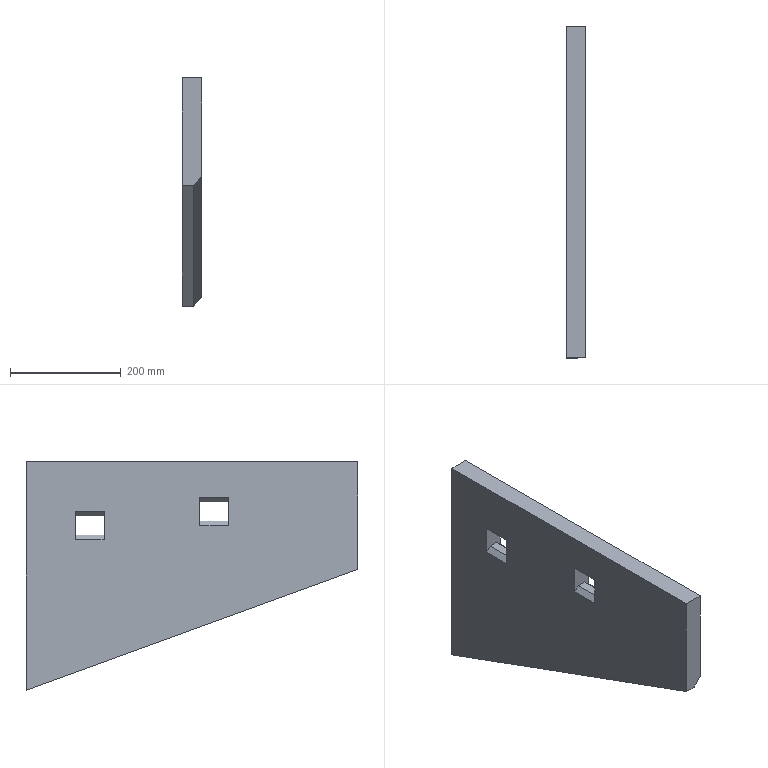Part | SolidWorks | features ICE 2, Chamfer 1, Extrusion 1 | 1 solid | 23 faces | box 35 x 600 x 413 mm | volume 6164844 mm3 | plane 23
STEP:
#1=CARTESIAN_POINT('',(2.5,-300.,-194.618));
#2=VERTEX_POINT('',#1);
#3=CARTESIAN_POINT('',(-17.5,-300.,-194.618));
#4=VERTEX_POINT('',#3);
#5=CARTESIAN_POINT('',(17.5,-300.,-194.618));
#6=DIRECTION('',(-1.,0.,0.));
#7=VECTOR('',#6,1000.);
#8=LINE('',#5,#7);
#9=EDGE_CURVE('',#2,#4,#8,.T.);
#10=ORIENTED_EDGE('',*,*,#9,.F.);
#11=CARTESIAN_POINT('',(17.5,-300.,-178.655));
#12=VERTEX_POINT('',#11);
#13=CARTESIAN_POINT('',(-20.187,-300.,-218.761));
#14=DIRECTION('',(0.6848,0.,0.7287));
#15=VECTOR('',#14,1000.);
#16=LINE('',#13,#15);
#17=EDGE_CURVE('',#2,#12,#16,.T.);
#18=ORIENTED_EDGE('',*,*,#17,.T.);
#19=CARTESIAN_POINT('',(17.5,-300.,0.));
#20=VERTEX_POINT('',#19);
#21=CARTESIAN_POINT('',(17.5,-300.,-194.618));
#22=DIRECTION('',(0.,0.,-1.));
#23=VECTOR('',#22,1000.);
#24=LINE('',#21,#23);
#25=EDGE_CURVE('',#20,#12,#24,.T.);
#26=ORIENTED_EDGE('',*,*,#25,.F.);
#27=CARTESIAN_POINT('',(-17.5,-300.,0.));
#28=VERTEX_POINT('',#27);
#29=CARTESIAN_POINT('',(17.5,-300.,0.));
#30=DIRECTION('',(-1.,0.,0.));
#31=VECTOR('',#30,1000.);
#32=LINE('',#29,#31);
#33=EDGE_CURVE('',#20,#28,#32,.T.);
#34=ORIENTED_EDGE('',*,*,#33,.T.);
#35=CARTESIAN_POINT('',(-17.5,-300.,-194.618));
#36=DIRECTION('',(0.,0.,-1.));
#37=VECTOR('',#36,1000.);
#38=LINE('',#35,#37);
#39=EDGE_CURVE('',#28,#4,#38,.T.);
#40=ORIENTED_EDGE('',*,*,#39,.T.);
#41=EDGE_LOOP('',(#10,#18,#26,#34,#40));
#42=FACE_OUTER_BOUND('',#41,.T.);
#43=CARTESIAN_POINT('',(17.5,-300.,-194.618));
#44=DIRECTION('',(0.,1.,0.));
#45=DIRECTION('',(0.,0.,1.));
#46=AXIS2_PLACEMENT_3D('',#43,#44,#45);
#47=PLANE('',#46);
#48=ADVANCED_FACE('',(#42),#47,.F.);
#49=CARTESIAN_POINT('',(2.5,300.,-413.));
#50=VERTEX_POINT('',#49);
#51=CARTESIAN_POINT('',(-17.5,300.,-413.));
#52=VERTEX_POINT('',#51);
#53=CARTESIAN_POINT('',(17.5,300.,-413.));
#54=DIRECTION('',(-1.,0.,0.));
#55=VECTOR('',#54,1000.);
#56=LINE('',#53,#55);
#57=EDGE_CURVE('',#50,#52,#56,.T.);
#58=ORIENTED_EDGE('',*,*,#57,.F.);
#59=CARTESIAN_POINT('',(2.5,300.,-413.));
#60=DIRECTION('',(0.,-0.9397,0.342));
#61=VECTOR('',#60,1000.);
#62=LINE('',#59,#61);
#63=EDGE_CURVE('',#50,#2,#62,.T.);
#64=ORIENTED_EDGE('',*,*,#63,.T.);
#65=ORIENTED_EDGE('',*,*,#9,.T.);
#66=CARTESIAN_POINT('',(-17.5,300.,-413.));
#67=DIRECTION('',(0.,0.9397,-0.342));
#68=VECTOR('',#67,1000.);
#69=LINE('',#66,#68);
#70=EDGE_CURVE('',#4,#52,#69,.T.);
#71=ORIENTED_EDGE('',*,*,#70,.T.);
#72=EDGE_LOOP('',(#58,#64,#65,#71));
#73=FACE_OUTER_BOUND('',#72,.T.);
#74=CARTESIAN_POINT('',(17.5,300.,-413.));
#75=DIRECTION('',(0.,0.342,0.9397));
#76=DIRECTION('',(0.,-0.9397,0.342));
#77=AXIS2_PLACEMENT_3D('',#74,#75,#76);
#78=PLANE('',#77);
#79=ADVANCED_FACE('',(#73),#78,.F.);
#80=CARTESIAN_POINT('',(17.5,300.,-397.037));
#81=VERTEX_POINT('',#80);
#82=CARTESIAN_POINT('',(17.5,300.,0.));
#83=VERTEX_POINT('',#82);
#84=CARTESIAN_POINT('',(17.5,300.,0.));
#85=DIRECTION('',(0.,0.,1.));
#86=VECTOR('',#85,1000.);
#87=LINE('',#84,#86);
#88=EDGE_CURVE('',#81,#83,#87,.T.);
#89=ORIENTED_EDGE('',*,*,#88,.F.);
#90=CARTESIAN_POINT('',(88.793,300.,-321.169));
#91=DIRECTION('',(-0.6848,0.,-0.7287));
#92=VECTOR('',#91,1000.);
#93=LINE('',#90,#92);
#94=EDGE_CURVE('',#81,#50,#93,.T.);
#95=ORIENTED_EDGE('',*,*,#94,.T.);
#96=ORIENTED_EDGE('',*,*,#57,.T.);
#97=CARTESIAN_POINT('',(-17.5,300.,0.));
#98=VERTEX_POINT('',#97);
#99=CARTESIAN_POINT('',(-17.5,300.,0.));
#100=DIRECTION('',(0.,0.,1.));
#101=VECTOR('',#100,1000.);
#102=LINE('',#99,#101);
#103=EDGE_CURVE('',#52,#98,#102,.T.);
#104=ORIENTED_EDGE('',*,*,#103,.T.);
#105=CARTESIAN_POINT('',(17.5,300.,0.));
#106=DIRECTION('',(-1.,0.,0.));
#107=VECTOR('',#106,1000.);
#108=LINE('',#105,#107);
#109=EDGE_CURVE('',#83,#98,#108,.T.);
#110=ORIENTED_EDGE('',*,*,#109,.F.);
#111=EDGE_LOOP('',(#89,#95,#96,#104,#110));
#112=FACE_OUTER_BOUND('',#111,.T.);
#113=CARTESIAN_POINT('',(17.5,300.,0.));
#114=DIRECTION('',(0.,-1.,0.));
#115=DIRECTION('',(0.,0.,-1.));
#116=AXIS2_PLACEMENT_3D('',#113,#114,#115);
#117=PLANE('',#116);
#118=ADVANCED_FACE('',(#112),#117,.F.);
#119=CARTESIAN_POINT('',(-17.5,0.,0.));
#120=DIRECTION('',(0.,-1.,0.));
#121=VECTOR('',#120,1000.);
#122=LINE('',#119,#121);
#123=EDGE_CURVE('',#98,#28,#122,.T.);
#124=ORIENTED_EDGE('',*,*,#123,.T.);
#125=ORIENTED_EDGE('',*,*,#33,.F.);
#126=CARTESIAN_POINT('',(17.5,-300.,0.));
#127=DIRECTION('',(0.,-1.,0.));
#128=VECTOR('',#127,1000.);
#129=LINE('',#126,#128);
#130=EDGE_CURVE('',#83,#20,#129,.T.);
#131=ORIENTED_EDGE('',*,*,#130,.F.);
#132=ORIENTED_EDGE('',*,*,#109,.T.);
#133=EDGE_LOOP('',(#124,#125,#131,#132));
#134=FACE_OUTER_BOUND('',#133,.T.);
#135=CARTESIAN_POINT('',(17.5,0.,0.));
#136=DIRECTION('',(0.,0.,-1.));
#137=DIRECTION('',(-1.,0.,0.));
#138=AXIS2_PLACEMENT_3D('',#135,#136,#137);
#139=PLANE('',#138);
#140=ADVANCED_FACE('',(#134),#139,.F.);
#141=CARTESIAN_POINT('',(17.5,-66.,-116.));
#142=VERTEX_POINT('',#141);
#143=CARTESIAN_POINT('',(17.5,-14.,-116.));
#144=VERTEX_POINT('',#143);
#145=CARTESIAN_POINT('',(17.5,-66.,-116.));
#146=DIRECTION('',(0.,1.,0.));
#147=VECTOR('',#146,1000.);
#148=LINE('',#145,#147);
#149=EDGE_CURVE('',#142,#144,#148,.T.);
#150=ORIENTED_EDGE('',*,*,#149,.F.);
#151=CARTESIAN_POINT('',(17.5,-66.,-64.));
#152=VERTEX_POINT('',#151);
#153=CARTESIAN_POINT('',(17.5,-66.,-64.));
#154=DIRECTION('',(0.,0.,-1.));
#155=VECTOR('',#154,1000.);
#156=LINE('',#153,#155);
#157=EDGE_CURVE('',#152,#142,#156,.T.);
#158=ORIENTED_EDGE('',*,*,#157,.F.);
#159=CARTESIAN_POINT('',(17.5,-14.,-64.));
#160=VERTEX_POINT('',#159);
#161=CARTESIAN_POINT('',(17.5,-66.,-64.));
#162=DIRECTION('',(0.,1.,0.));
#163=VECTOR('',#162,1000.);
#164=LINE('',#161,#163);
#165=EDGE_CURVE('',#152,#160,#164,.T.);
#166=ORIENTED_EDGE('',*,*,#165,.T.);
#167=CARTESIAN_POINT('',(17.5,-14.,-64.));
#168=DIRECTION('',(0.,0.,-1.));
#169=VECTOR('',#168,1000.);
#170=LINE('',#167,#169);
#171=EDGE_CURVE('',#160,#144,#170,.T.);
#172=ORIENTED_EDGE('',*,*,#171,.T.);
#173=EDGE_LOOP('',(#150,#158,#166,#172));
#174=FACE_BOUND('',#173,.T.);
#175=CARTESIAN_POINT('',(17.5,159.,-141.));
#176=VERTEX_POINT('',#175);
#177=CARTESIAN_POINT('',(17.5,211.,-141.));
#178=VERTEX_POINT('',#177);
#179=CARTESIAN_POINT('',(17.5,159.,-141.));
#180=DIRECTION('',(0.,1.,0.));
#181=VECTOR('',#180,1000.);
#182=LINE('',#179,#181);
#183=EDGE_CURVE('',#176,#178,#182,.T.);
#184=ORIENTED_EDGE('',*,*,#183,.F.);
#185=CARTESIAN_POINT('',(17.5,159.,-89.));
#186=VERTEX_POINT('',#185);
#187=CARTESIAN_POINT('',(17.5,159.,-89.));
#188=DIRECTION('',(0.,0.,-1.));
#189=VECTOR('',#188,1000.);
#190=LINE('',#187,#189);
#191=EDGE_CURVE('',#186,#176,#190,.T.);
#192=ORIENTED_EDGE('',*,*,#191,.F.);
#193=CARTESIAN_POINT('',(17.5,211.,-89.));
#194=VERTEX_POINT('',#193);
#195=CARTESIAN_POINT('',(17.5,159.,-89.));
#196=DIRECTION('',(0.,1.,0.));
#197=VECTOR('',#196,1000.);
#198=LINE('',#195,#197);
#199=EDGE_CURVE('',#186,#194,#198,.T.);
#200=ORIENTED_EDGE('',*,*,#199,.T.);
#201=CARTESIAN_POINT('',(17.5,211.,-89.));
#202=DIRECTION('',(0.,0.,-1.));
#203=VECTOR('',#202,1000.);
#204=LINE('',#201,#203);
#205=EDGE_CURVE('',#194,#178,#204,.T.);
#206=ORIENTED_EDGE('',*,*,#205,.T.);
#207=EDGE_LOOP('',(#184,#192,#200,#206));
#208=FACE_BOUND('',#207,.T.);
#209=ORIENTED_EDGE('',*,*,#25,.T.);
#210=CARTESIAN_POINT('',(17.5,-92.512,-254.175));
#211=DIRECTION('',(0.,0.9397,-0.342));
#212=VECTOR('',#211,1000.);
#213=LINE('',#210,#212);
#214=EDGE_CURVE('',#12,#81,#213,.T.);
#215=ORIENTED_EDGE('',*,*,#214,.T.);
#216=ORIENTED_EDGE('',*,*,#88,.T.);
#217=ORIENTED_EDGE('',*,*,#130,.T.);
#218=EDGE_LOOP('',(#209,#215,#216,#217));
#219=FACE_OUTER_BOUND('',#218,.T.);
#220=CARTESIAN_POINT('',(17.5,0.,0.));
#221=DIRECTION('',(-1.,0.,0.));
#222=DIRECTION('',(0.,0.,1.));
#223=AXIS2_PLACEMENT_3D('',#220,#221,#222);
#224=PLANE('',#223);
#225=ADVANCED_FACE('',(#174,#208,#219),#224,.F.);
#226=CARTESIAN_POINT('',(-17.5,-66.,-116.));
#227=VERTEX_POINT('',#226);
#228=CARTESIAN_POINT('',(-17.5,-66.,-64.));
#229=VERTEX_POINT('',#228);
#230=CARTESIAN_POINT('',(-17.5,-66.,-64.));
#231=DIRECTION('',(0.,0.,1.));
#232=VECTOR('',#231,1000.);
#233=LINE('',#230,#232);
#234=EDGE_CURVE('',#227,#229,#233,.T.);
#235=ORIENTED_EDGE('',*,*,#234,.F.);
#236=CARTESIAN_POINT('',(-17.5,-14.,-116.));
#237=VERTEX_POINT('',#236);
#238=CARTESIAN_POINT('',(-17.5,-66.,-116.));
#239=DIRECTION('',(0.,1.,0.));
#240=VECTOR('',#239,1000.);
#241=LINE('',#238,#240);
#242=EDGE_CURVE('',#227,#237,#241,.T.);
#243=ORIENTED_EDGE('',*,*,#242,.T.);
#244=CARTESIAN_POINT('',(-17.5,-14.,-64.));
#245=VERTEX_POINT('',#244);
#246=CARTESIAN_POINT('',(-17.5,-14.,-64.));
#247=DIRECTION('',(0.,0.,1.));
#248=VECTOR('',#247,1000.);
#249=LINE('',#246,#248);
#250=EDGE_CURVE('',#237,#245,#249,.T.);
#251=ORIENTED_EDGE('',*,*,#250,.T.);
#252=CARTESIAN_POINT('',(-17.5,-66.,-64.));
#253=DIRECTION('',(0.,1.,0.));
#254=VECTOR('',#253,1000.);
#255=LINE('',#252,#254);
#256=EDGE_CURVE('',#229,#245,#255,.T.);
#257=ORIENTED_EDGE('',*,*,#256,.F.);
#258=EDGE_LOOP('',(#235,#243,#251,#257));
#259=FACE_BOUND('',#258,.T.);
#260=CARTESIAN_POINT('',(-17.5,159.,-141.));
#261=VERTEX_POINT('',#260);
#262=CARTESIAN_POINT('',(-17.5,159.,-89.));
#263=VERTEX_POINT('',#262);
#264=CARTESIAN_POINT('',(-17.5,159.,-89.));
#265=DIRECTION('',(0.,0.,1.));
#266=VECTOR('',#265,1000.);
#267=LINE('',#264,#266);
#268=EDGE_CURVE('',#261,#263,#267,.T.);
#269=ORIENTED_EDGE('',*,*,#268,.F.);
#270=CARTESIAN_POINT('',(-17.5,211.,-141.));
#271=VERTEX_POINT('',#270);
#272=CARTESIAN_POINT('',(-17.5,159.,-141.));
#273=DIRECTION('',(0.,1.,0.));
#274=VECTOR('',#273,1000.);
#275=LINE('',#272,#274);
#276=EDGE_CURVE('',#261,#271,#275,.T.);
#277=ORIENTED_EDGE('',*,*,#276,.T.);
#278=CARTESIAN_POINT('',(-17.5,211.,-89.));
#279=VERTEX_POINT('',#278);
#280=CARTESIAN_POINT('',(-17.5,211.,-89.));
#281=DIRECTION('',(0.,0.,1.));
#282=VECTOR('',#281,1000.);
#283=LINE('',#280,#282);
#284=EDGE_CURVE('',#271,#279,#283,.T.);
#285=ORIENTED_EDGE('',*,*,#284,.T.);
#286=CARTESIAN_POINT('',(-17.5,159.,-89.));
#287=DIRECTION('',(0.,1.,0.));
#288=VECTOR('',#287,1000.);
#289=LINE('',#286,#288);
#290=EDGE_CURVE('',#263,#279,#289,.T.);
#291=ORIENTED_EDGE('',*,*,#290,.F.);
#292=EDGE_LOOP('',(#269,#277,#285,#291));
#293=FACE_BOUND('',#292,.T.);
#294=ORIENTED_EDGE('',*,*,#39,.F.);
#295=ORIENTED_EDGE('',*,*,#123,.F.);
#296=ORIENTED_EDGE('',*,*,#103,.F.);
#297=ORIENTED_EDGE('',*,*,#70,.F.);
#298=EDGE_LOOP('',(#294,#295,#296,#297));
#299=FACE_OUTER_BOUND('',#298,.T.);
#300=CARTESIAN_POINT('',(-17.5,0.,0.));
#301=DIRECTION('',(-1.,0.,0.));
#302=DIRECTION('',(0.,0.,1.));
#303=AXIS2_PLACEMENT_3D('',#300,#301,#302);
#304=PLANE('',#303);
#305=ADVANCED_FACE('',(#259,#293,#299),#304,.T.);
#306=CARTESIAN_POINT('',(-8.5,211.,-132.5));
#307=VERTEX_POINT('',#306);
#308=CARTESIAN_POINT('',(-17.5,211.,-141.));
#309=DIRECTION('',(-0.727,0.,-0.6866));
#310=VECTOR('',#309,1000.);
#311=LINE('',#308,#310);
#312=EDGE_CURVE('',#307,#271,#311,.T.);
#313=ORIENTED_EDGE('',*,*,#312,.T.);
#314=ORIENTED_EDGE('',*,*,#276,.F.);
#315=CARTESIAN_POINT('',(-8.5,159.,-132.5));
#316=VERTEX_POINT('',#315);
#317=CARTESIAN_POINT('',(-17.5,159.,-141.));
#318=DIRECTION('',(-0.727,0.,-0.6866));
#319=VECTOR('',#318,1000.);
#320=LINE('',#317,#319);
#321=EDGE_CURVE('',#316,#261,#320,.T.);
#322=ORIENTED_EDGE('',*,*,#321,.F.);
#323=CARTESIAN_POINT('',(-8.5,159.,-132.5));
#324=DIRECTION('',(0.,1.,0.));
#325=VECTOR('',#324,1000.);
#326=LINE('',#323,#325);
#327=EDGE_CURVE('',#316,#307,#326,.T.);
#328=ORIENTED_EDGE('',*,*,#327,.T.);
#329=EDGE_LOOP('',(#313,#314,#322,#328));
#330=FACE_OUTER_BOUND('',#329,.T.);
#331=CARTESIAN_POINT('',(-17.5,159.,-141.));
#332=DIRECTION('',(0.6866,0.,-0.727));
#333=DIRECTION('',(-0.727,0.,-0.6866));
#334=AXIS2_PLACEMENT_3D('',#331,#332,#333);
#335=PLANE('',#334);
#336=ADVANCED_FACE('',(#330),#335,.F.);
#337=CARTESIAN_POINT('',(8.5,211.,-132.5));
#338=VERTEX_POINT('',#337);
#339=CARTESIAN_POINT('',(-8.5,211.,-132.5));
#340=DIRECTION('',(-1.,0.,0.));
#341=VECTOR('',#340,1000.);
#342=LINE('',#339,#341);
#343=EDGE_CURVE('',#338,#307,#342,.T.);
#344=ORIENTED_EDGE('',*,*,#343,.T.);
#345=ORIENTED_EDGE('',*,*,#327,.F.);
#346=CARTESIAN_POINT('',(8.5,159.,-132.5));
#347=VERTEX_POINT('',#346);
#348=CARTESIAN_POINT('',(-8.5,159.,-132.5));
#349=DIRECTION('',(-1.,0.,0.));
#350=VECTOR('',#349,1000.);
#351=LINE('',#348,#350);
#352=EDGE_CURVE('',#347,#316,#351,.T.);
#353=ORIENTED_EDGE('',*,*,#352,.F.);
#354=CARTESIAN_POINT('',(8.5,159.,-132.5));
#355=DIRECTION('',(0.,1.,0.));
#356=VECTOR('',#355,1000.);
#357=LINE('',#354,#356);
#358=EDGE_CURVE('',#347,#338,#357,.T.);
#359=ORIENTED_EDGE('',*,*,#358,.T.);
#360=EDGE_LOOP('',(#344,#345,#353,#359));
#361=FACE_OUTER_BOUND('',#360,.T.);
#362=CARTESIAN_POINT('',(-8.5,159.,-132.5));
#363=DIRECTION('',(0.,0.,-1.));
#364=DIRECTION('',(-1.,0.,0.));
#365=AXIS2_PLACEMENT_3D('',#362,#363,#364);
#366=PLANE('',#365);
#367=ADVANCED_FACE('',(#361),#366,.F.);
#368=CARTESIAN_POINT('',(8.5,211.,-132.5));
#369=DIRECTION('',(-0.727,0.,0.6866));
#370=VECTOR('',#369,1000.);
#371=LINE('',#368,#370);
#372=EDGE_CURVE('',#178,#338,#371,.T.);
#373=ORIENTED_EDGE('',*,*,#372,.T.);
#374=ORIENTED_EDGE('',*,*,#358,.F.);
#375=CARTESIAN_POINT('',(8.5,159.,-132.5));
#376=DIRECTION('',(-0.727,0.,0.6866));
#377=VECTOR('',#376,1000.);
#378=LINE('',#375,#377);
#379=EDGE_CURVE('',#176,#347,#378,.T.);
#380=ORIENTED_EDGE('',*,*,#379,.F.);
#381=ORIENTED_EDGE('',*,*,#183,.T.);
#382=EDGE_LOOP('',(#373,#374,#380,#381));
#383=FACE_OUTER_BOUND('',#382,.T.);
#384=CARTESIAN_POINT('',(8.5,159.,-132.5));
#385=DIRECTION('',(-0.6866,0.,-0.727));
#386=DIRECTION('',(-0.727,0.,0.6866));
#387=AXIS2_PLACEMENT_3D('',#384,#385,#386);
#388=PLANE('',#387);
#389=ADVANCED_FACE('',(#383),#388,.F.);
#390=CARTESIAN_POINT('',(8.5,211.,-97.5));
#391=VERTEX_POINT('',#390);
#392=CARTESIAN_POINT('',(8.5,211.,-97.5));
#393=DIRECTION('',(0.727,0.,0.6866));
#394=VECTOR('',#393,1000.);
#395=LINE('',#392,#394);
#396=EDGE_CURVE('',#391,#194,#395,.T.);
#397=ORIENTED_EDGE('',*,*,#396,.T.);
#398=ORIENTED_EDGE('',*,*,#199,.F.);
#399=CARTESIAN_POINT('',(8.5,159.,-97.5));
#400=VERTEX_POINT('',#399);
#401=CARTESIAN_POINT('',(8.5,159.,-97.5));
#402=DIRECTION('',(0.727,0.,0.6866));
#403=VECTOR('',#402,1000.);
#404=LINE('',#401,#403);
#405=EDGE_CURVE('',#400,#186,#404,.T.);
#406=ORIENTED_EDGE('',*,*,#405,.F.);
#407=CARTESIAN_POINT('',(8.5,159.,-97.5));
#408=DIRECTION('',(0.,1.,0.));
#409=VECTOR('',#408,1000.);
#410=LINE('',#407,#409);
#411=EDGE_CURVE('',#400,#391,#410,.T.);
#412=ORIENTED_EDGE('',*,*,#411,.T.);
#413=EDGE_LOOP('',(#397,#398,#406,#412));
#414=FACE_OUTER_BOUND('',#413,.T.);
#415=CARTESIAN_POINT('',(8.5,159.,-97.5));
#416=DIRECTION('',(-0.6866,0.,0.727));
#417=DIRECTION('',(0.727,0.,0.6866));
#418=AXIS2_PLACEMENT_3D('',#415,#416,#417);
#419=PLANE('',#418);
#420=ADVANCED_FACE('',(#414),#419,.F.);
#421=CARTESIAN_POINT('',(-8.5,211.,-97.5));
#422=VERTEX_POINT('',#421);
#423=CARTESIAN_POINT('',(-8.5,211.,-97.5));
#424=DIRECTION('',(1.,0.,0.));
#425=VECTOR('',#424,1000.);
#426=LINE('',#423,#425);
#427=EDGE_CURVE('',#422,#391,#426,.T.);
#428=ORIENTED_EDGE('',*,*,#427,.T.);
#429=ORIENTED_EDGE('',*,*,#411,.F.);
#430=CARTESIAN_POINT('',(-8.5,159.,-97.5));
#431=VERTEX_POINT('',#430);
#432=CARTESIAN_POINT('',(-8.5,159.,-97.5));
#433=DIRECTION('',(1.,0.,0.));
#434=VECTOR('',#433,1000.);
#435=LINE('',#432,#434);
#436=EDGE_CURVE('',#431,#400,#435,.T.);
#437=ORIENTED_EDGE('',*,*,#436,.F.);
#438=CARTESIAN_POINT('',(-8.5,159.,-97.5));
#439=DIRECTION('',(0.,1.,0.));
#440=VECTOR('',#439,1000.);
#441=LINE('',#438,#440);
#442=EDGE_CURVE('',#431,#422,#441,.T.);
#443=ORIENTED_EDGE('',*,*,#442,.T.);
#444=EDGE_LOOP('',(#428,#429,#437,#443));
#445=FACE_OUTER_BOUND('',#444,.T.);
#446=CARTESIAN_POINT('',(-8.5,159.,-97.5));
#447=DIRECTION('',(0.,0.,1.));
#448=DIRECTION('',(1.,0.,0.));
#449=AXIS2_PLACEMENT_3D('',#446,#447,#448);
#450=PLANE('',#449);
#451=ADVANCED_FACE('',(#445),#450,.F.);
#452=CARTESIAN_POINT('',(-17.5,211.,-89.));
#453=DIRECTION('',(0.727,0.,-0.6866));
#454=VECTOR('',#453,1000.);
#455=LINE('',#452,#454);
#456=EDGE_CURVE('',#279,#422,#455,.T.);
#457=ORIENTED_EDGE('',*,*,#456,.T.);
#458=ORIENTED_EDGE('',*,*,#442,.F.);
#459=CARTESIAN_POINT('',(-17.5,159.,-89.));
#460=DIRECTION('',(0.727,0.,-0.6866));
#461=VECTOR('',#460,1000.);
#462=LINE('',#459,#461);
#463=EDGE_CURVE('',#263,#431,#462,.T.);
#464=ORIENTED_EDGE('',*,*,#463,.F.);
#465=ORIENTED_EDGE('',*,*,#290,.T.);
#466=EDGE_LOOP('',(#457,#458,#464,#465));
#467=FACE_OUTER_BOUND('',#466,.T.);
#468=CARTESIAN_POINT('',(-17.5,159.,-89.));
#469=DIRECTION('',(0.6866,0.,0.727));
#470=DIRECTION('',(0.727,0.,-0.6866));
#471=AXIS2_PLACEMENT_3D('',#468,#469,#470);
#472=PLANE('',#471);
#473=ADVANCED_FACE('',(#467),#472,.F.);
#474=ORIENTED_EDGE('',*,*,#268,.T.);
#475=ORIENTED_EDGE('',*,*,#463,.T.);
#476=ORIENTED_EDGE('',*,*,#436,.T.);
#477=ORIENTED_EDGE('',*,*,#405,.T.);
#478=ORIENTED_EDGE('',*,*,#191,.T.);
#479=ORIENTED_EDGE('',*,*,#379,.T.);
#480=ORIENTED_EDGE('',*,*,#352,.T.);
#481=ORIENTED_EDGE('',*,*,#321,.T.);
#482=EDGE_LOOP('',(#474,#475,#476,#477,#478,#479,#480,#481));
#483=FACE_OUTER_BOUND('',#482,.T.);
#484=CARTESIAN_POINT('',(0.,159.,0.));
#485=DIRECTION('',(0.,-1.,0.));
#486=DIRECTION('',(0.,0.,-1.));
#487=AXIS2_PLACEMENT_3D('',#484,#485,#486);
#488=PLANE('',#487);
#489=ADVANCED_FACE('',(#483),#488,.F.);
#490=ORIENTED_EDGE('',*,*,#284,.F.);
#491=ORIENTED_EDGE('',*,*,#312,.F.);
#492=ORIENTED_EDGE('',*,*,#343,.F.);
#493=ORIENTED_EDGE('',*,*,#372,.F.);
#494=ORIENTED_EDGE('',*,*,#205,.F.);
#495=ORIENTED_EDGE('',*,*,#396,.F.);
#496=ORIENTED_EDGE('',*,*,#427,.F.);
#497=ORIENTED_EDGE('',*,*,#456,.F.);
#498=EDGE_LOOP('',(#490,#491,#492,#493,#494,#495,#496,#497));
#499=FACE_OUTER_BOUND('',#498,.T.);
#500=CARTESIAN_POINT('',(0.,211.,0.));
#501=DIRECTION('',(0.,-1.,0.));
#502=DIRECTION('',(0.,0.,-1.));
#503=AXIS2_PLACEMENT_3D('',#500,#501,#502);
#504=PLANE('',#503);
#505=ADVANCED_FACE('',(#499),#504,.T.);
#506=ORIENTED_EDGE('',*,*,#17,.F.);
#507=ORIENTED_EDGE('',*,*,#63,.F.);
#508=ORIENTED_EDGE('',*,*,#94,.F.);
#509=ORIENTED_EDGE('',*,*,#214,.F.);
#510=EDGE_LOOP('',(#506,#507,#508,#509));
#511=FACE_OUTER_BOUND('',#510,.T.);
#512=CARTESIAN_POINT('',(17.5,-92.512,-254.175));
#513=DIRECTION('',(-0.7071,0.2418,0.6645));
#514=DIRECTION('',(0.,0.9397,-0.342));
#515=AXIS2_PLACEMENT_3D('',#512,#513,#514);
#516=PLANE('',#515);
#517=ADVANCED_FACE('',(#511),#516,.F.);
#518=CARTESIAN_POINT('',(-8.5,-14.,-107.5));
#519=VERTEX_POINT('',#518);
#520=CARTESIAN_POINT('',(-17.5,-14.,-116.));
#521=DIRECTION('',(-0.727,0.,-0.6866));
#522=VECTOR('',#521,1000.);
#523=LINE('',#520,#522);
#524=EDGE_CURVE('',#519,#237,#523,.T.);
#525=ORIENTED_EDGE('',*,*,#524,.T.);
#526=ORIENTED_EDGE('',*,*,#242,.F.);
#527=CARTESIAN_POINT('',(-8.5,-66.,-107.5));
#528=VERTEX_POINT('',#527);
#529=CARTESIAN_POINT('',(-17.5,-66.,-116.));
#530=DIRECTION('',(-0.727,0.,-0.6866));
#531=VECTOR('',#530,1000.);
#532=LINE('',#529,#531);
#533=EDGE_CURVE('',#528,#227,#532,.T.);
#534=ORIENTED_EDGE('',*,*,#533,.F.);
#535=CARTESIAN_POINT('',(-8.5,-66.,-107.5));
#536=DIRECTION('',(0.,1.,0.));
#537=VECTOR('',#536,1000.);
#538=LINE('',#535,#537);
#539=EDGE_CURVE('',#528,#519,#538,.T.);
#540=ORIENTED_EDGE('',*,*,#539,.T.);
#541=EDGE_LOOP('',(#525,#526,#534,#540));
#542=FACE_OUTER_BOUND('',#541,.T.);
#543=CARTESIAN_POINT('',(-17.5,-66.,-116.));
#544=DIRECTION('',(0.6866,0.,-0.727));
#545=DIRECTION('',(-0.727,0.,-0.6866));
#546=AXIS2_PLACEMENT_3D('',#543,#544,#545);
#547=PLANE('',#546);
#548=ADVANCED_FACE('',(#542),#547,.F.);
#549=CARTESIAN_POINT('',(8.5,-14.,-107.5));
#550=VERTEX_POINT('',#549);
#551=CARTESIAN_POINT('',(-8.5,-14.,-107.5));
#552=DIRECTION('',(-1.,0.,0.));
#553=VECTOR('',#552,1000.);
#554=LINE('',#551,#553);
#555=EDGE_CURVE('',#550,#519,#554,.T.);
#556=ORIENTED_EDGE('',*,*,#555,.T.);
#557=ORIENTED_EDGE('',*,*,#539,.F.);
#558=CARTESIAN_POINT('',(8.5,-66.,-107.5));
#559=VERTEX_POINT('',#558);
#560=CARTESIAN_POINT('',(-8.5,-66.,-107.5));
#561=DIRECTION('',(-1.,0.,0.));
#562=VECTOR('',#561,1000.);
#563=LINE('',#560,#562);
#564=EDGE_CURVE('',#559,#528,#563,.T.);
#565=ORIENTED_EDGE('',*,*,#564,.F.);
#566=CARTESIAN_POINT('',(8.5,-66.,-107.5));
#567=DIRECTION('',(0.,1.,0.));
#568=VECTOR('',#567,1000.);
#569=LINE('',#566,#568);
#570=EDGE_CURVE('',#559,#550,#569,.T.);
#571=ORIENTED_EDGE('',*,*,#570,.T.);
#572=EDGE_LOOP('',(#556,#557,#565,#571));
#573=FACE_OUTER_BOUND('',#572,.T.);
#574=CARTESIAN_POINT('',(-8.5,-66.,-107.5));
#575=DIRECTION('',(0.,0.,-1.));
#576=DIRECTION('',(-1.,0.,0.));
#577=AXIS2_PLACEMENT_3D('',#574,#575,#576);
#578=PLANE('',#577);
#579=ADVANCED_FACE('',(#573),#578,.F.);
#580=CARTESIAN_POINT('',(8.5,-14.,-107.5));
#581=DIRECTION('',(-0.727,0.,0.6866));
#582=VECTOR('',#581,1000.);
#583=LINE('',#580,#582);
#584=EDGE_CURVE('',#144,#550,#583,.T.);
#585=ORIENTED_EDGE('',*,*,#584,.T.);
#586=ORIENTED_EDGE('',*,*,#570,.F.);
#587=CARTESIAN_POINT('',(8.5,-66.,-107.5));
#588=DIRECTION('',(-0.727,0.,0.6866));
#589=VECTOR('',#588,1000.);
#590=LINE('',#587,#589);
#591=EDGE_CURVE('',#142,#559,#590,.T.);
#592=ORIENTED_EDGE('',*,*,#591,.F.);
#593=ORIENTED_EDGE('',*,*,#149,.T.);
#594=EDGE_LOOP('',(#585,#586,#592,#593));
#595=FACE_OUTER_BOUND('',#594,.T.);
#596=CARTESIAN_POINT('',(8.5,-66.,-107.5));
#597=DIRECTION('',(-0.6866,0.,-0.727));
#598=DIRECTION('',(-0.727,0.,0.6866));
#599=AXIS2_PLACEMENT_3D('',#596,#597,#598);
#600=PLANE('',#599);
#601=ADVANCED_FACE('',(#595),#600,.F.);
#602=CARTESIAN_POINT('',(8.5,-14.,-72.5));
#603=VERTEX_POINT('',#602);
#604=CARTESIAN_POINT('',(8.5,-14.,-72.5));
#605=DIRECTION('',(0.727,0.,0.6866));
#606=VECTOR('',#605,1000.);
#607=LINE('',#604,#606);
#608=EDGE_CURVE('',#603,#160,#607,.T.);
#609=ORIENTED_EDGE('',*,*,#608,.T.);
#610=ORIENTED_EDGE('',*,*,#165,.F.);
#611=CARTESIAN_POINT('',(8.5,-66.,-72.5));
#612=VERTEX_POINT('',#611);
#613=CARTESIAN_POINT('',(8.5,-66.,-72.5));
#614=DIRECTION('',(0.727,0.,0.6866));
#615=VECTOR('',#614,1000.);
#616=LINE('',#613,#615);
#617=EDGE_CURVE('',#612,#152,#616,.T.);
#618=ORIENTED_EDGE('',*,*,#617,.F.);
#619=CARTESIAN_POINT('',(8.5,-66.,-72.5));
#620=DIRECTION('',(0.,1.,0.));
#621=VECTOR('',#620,1000.);
#622=LINE('',#619,#621);
#623=EDGE_CURVE('',#612,#603,#622,.T.);
#624=ORIENTED_EDGE('',*,*,#623,.T.);
#625=EDGE_LOOP('',(#609,#610,#618,#624));
#626=FACE_OUTER_BOUND('',#625,.T.);
#627=CARTESIAN_POINT('',(8.5,-66.,-72.5));
#628=DIRECTION('',(-0.6866,0.,0.727));
#629=DIRECTION('',(0.727,0.,0.6866));
#630=AXIS2_PLACEMENT_3D('',#627,#628,#629);
#631=PLANE('',#630);
#632=ADVANCED_FACE('',(#626),#631,.F.);
#633=CARTESIAN_POINT('',(-8.5,-14.,-72.5));
#634=VERTEX_POINT('',#633);
#635=CARTESIAN_POINT('',(-8.5,-14.,-72.5));
#636=DIRECTION('',(1.,0.,0.));
#637=VECTOR('',#636,1000.);
#638=LINE('',#635,#637);
#639=EDGE_CURVE('',#634,#603,#638,.T.);
#640=ORIENTED_EDGE('',*,*,#639,.T.);
#641=ORIENTED_EDGE('',*,*,#623,.F.);
#642=CARTESIAN_POINT('',(-8.5,-66.,-72.5));
#643=VERTEX_POINT('',#642);
#644=CARTESIAN_POINT('',(-8.5,-66.,-72.5));
#645=DIRECTION('',(1.,0.,0.));
#646=VECTOR('',#645,1000.);
#647=LINE('',#644,#646);
#648=EDGE_CURVE('',#643,#612,#647,.T.);
#649=ORIENTED_EDGE('',*,*,#648,.F.);
#650=CARTESIAN_POINT('',(-8.5,-66.,-72.5));
#651=DIRECTION('',(0.,1.,0.));
#652=VECTOR('',#651,1000.);
#653=LINE('',#650,#652);
#654=EDGE_CURVE('',#643,#634,#653,.T.);
#655=ORIENTED_EDGE('',*,*,#654,.T.);
#656=EDGE_LOOP('',(#640,#641,#649,#655));
#657=FACE_OUTER_BOUND('',#656,.T.);
#658=CARTESIAN_POINT('',(-8.5,-66.,-72.5));
#659=DIRECTION('',(0.,0.,1.));
#660=DIRECTION('',(1.,0.,0.));
#661=AXIS2_PLACEMENT_3D('',#658,#659,#660);
#662=PLANE('',#661);
#663=ADVANCED_FACE('',(#657),#662,.F.);
#664=CARTESIAN_POINT('',(-17.5,-14.,-64.));
#665=DIRECTION('',(0.727,0.,-0.6866));
#666=VECTOR('',#665,1000.);
#667=LINE('',#664,#666);
#668=EDGE_CURVE('',#245,#634,#667,.T.);
#669=ORIENTED_EDGE('',*,*,#668,.T.);
#670=ORIENTED_EDGE('',*,*,#654,.F.);
#671=CARTESIAN_POINT('',(-17.5,-66.,-64.));
#672=DIRECTION('',(0.727,0.,-0.6866));
#673=VECTOR('',#672,1000.);
#674=LINE('',#671,#673);
#675=EDGE_CURVE('',#229,#643,#674,.T.);
#676=ORIENTED_EDGE('',*,*,#675,.F.);
#677=ORIENTED_EDGE('',*,*,#256,.T.);
#678=EDGE_LOOP('',(#669,#670,#676,#677));
#679=FACE_OUTER_BOUND('',#678,.T.);
#680=CARTESIAN_POINT('',(-17.5,-66.,-64.));
#681=DIRECTION('',(0.6866,0.,0.727));
#682=DIRECTION('',(0.727,0.,-0.6866));
#683=AXIS2_PLACEMENT_3D('',#680,#681,#682);
#684=PLANE('',#683);
#685=ADVANCED_FACE('',(#679),#684,.F.);
#686=ORIENTED_EDGE('',*,*,#234,.T.);
#687=ORIENTED_EDGE('',*,*,#675,.T.);
#688=ORIENTED_EDGE('',*,*,#648,.T.);
#689=ORIENTED_EDGE('',*,*,#617,.T.);
#690=ORIENTED_EDGE('',*,*,#157,.T.);
#691=ORIENTED_EDGE('',*,*,#591,.T.);
#692=ORIENTED_EDGE('',*,*,#564,.T.);
#693=ORIENTED_EDGE('',*,*,#533,.T.);
#694=EDGE_LOOP('',(#686,#687,#688,#689,#690,#691,#692,#693));
#695=FACE_OUTER_BOUND('',#694,.T.);
#696=CARTESIAN_POINT('',(0.,-66.,0.));
#697=DIRECTION('',(0.,-1.,0.));
#698=DIRECTION('',(0.,0.,-1.));
#699=AXIS2_PLACEMENT_3D('',#696,#697,#698);
#700=PLANE('',#699);
#701=ADVANCED_FACE('',(#695),#700,.F.);
#702=ORIENTED_EDGE('',*,*,#250,.F.);
#703=ORIENTED_EDGE('',*,*,#524,.F.);
#704=ORIENTED_EDGE('',*,*,#555,.F.);
#705=ORIENTED_EDGE('',*,*,#584,.F.);
#706=ORIENTED_EDGE('',*,*,#171,.F.);
#707=ORIENTED_EDGE('',*,*,#608,.F.);
#708=ORIENTED_EDGE('',*,*,#639,.F.);
#709=ORIENTED_EDGE('',*,*,#668,.F.);
#710=EDGE_LOOP('',(#702,#703,#704,#705,#706,#707,#708,#709));
#711=FACE_OUTER_BOUND('',#710,.T.);
#712=CARTESIAN_POINT('',(0.,-14.,0.));
#713=DIRECTION('',(0.,-1.,0.));
#714=DIRECTION('',(0.,0.,-1.));
#715=AXIS2_PLACEMENT_3D('',#712,#713,#714);
#716=PLANE('',#715);
#717=ADVANCED_FACE('',(#711),#716,.T.);
#718=CLOSED_SHELL('',(#48,#79,#118,#140,#225,#305,#336,#367,#389,#420,#451,#473,#489,#505,#517,#548,#579,#601,#632,#663,#685,#701,#717));
#719=MANIFOLD_SOLID_BREP('',#718);
#720=CARTESIAN_POINT('',(0.,0.,0.));
#721=DIRECTION('',(0.,0.,1.));
#722=DIRECTION('',(1.,0.,0.));
#723=AXIS2_PLACEMENT_3D('',#720,#721,#722);
#724=(LENGTH_UNIT()NAMED_UNIT(*)SI_UNIT(.MILLI.,.METRE.));
#725=UNCERTAINTY_MEASURE_WITH_UNIT(LENGTH_MEASURE(0.00001),#724,'','');
#726=(NAMED_UNIT(*)PLANE_ANGLE_UNIT()SI_UNIT($,.RADIAN.));
#727=(NAMED_UNIT(*)SI_UNIT($,.STERADIAN.)SOLID_ANGLE_UNIT());
#728=(GEOMETRIC_REPRESENTATION_CONTEXT(3)GLOBAL_UNCERTAINTY_ASSIGNED_CONTEXT((#725))GLOBAL_UNIT_ASSIGNED_CONTEXT((#724,#726,#727))REPRESENTATION_CONTEXT('',''));
#729=ADVANCED_BREP_SHAPE_REPRESENTATION('',(#719,#723),#728);